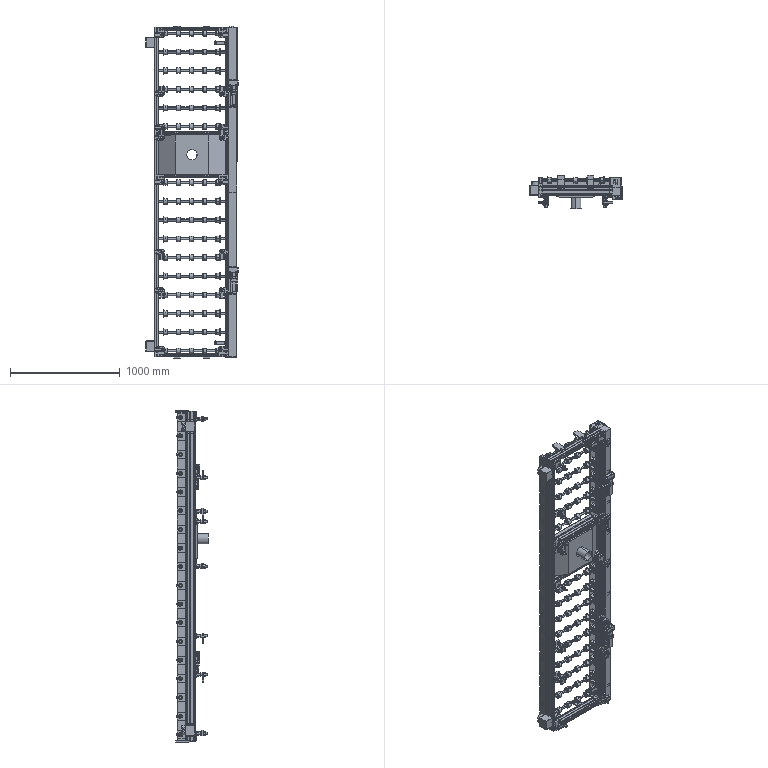Part | SolidWorks | 507 solids | 14621 faces | volume 44300991 mm3 | cylinder 7256 | plane 4914 | cone 1363 | sphere 608 | torus 406 | spline 74 | commonest cylinder face diameters 4 x978 18 x800 4.2 x636 20 x556 6.6 x382 0.8 x364